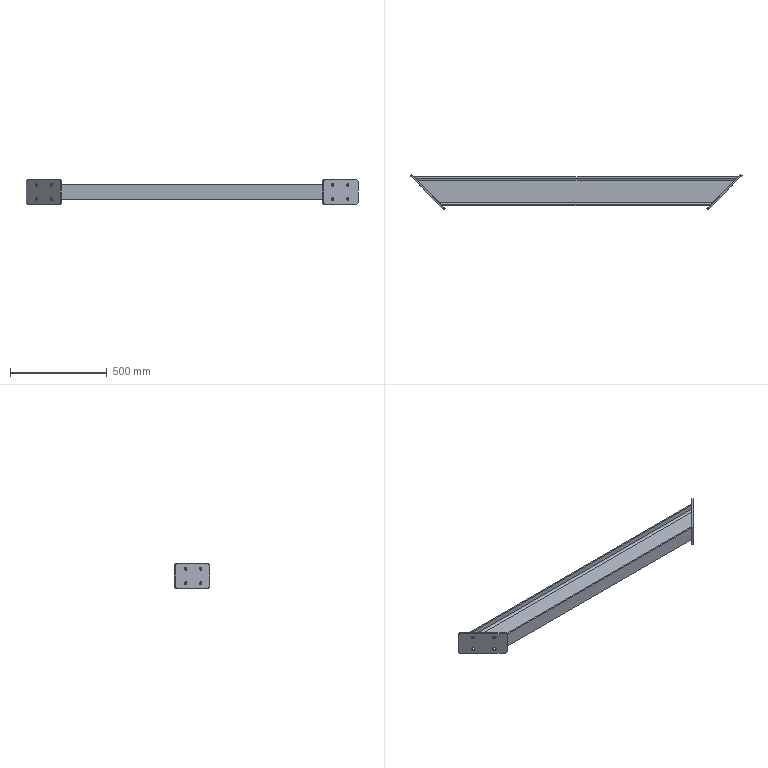Part | STEP file | PN_0059 steel column and steel beam brace 1677_Default<As Machined> | 3 solids | 46 faces | box 1715 x 182.434 x 125 mm | volume 3255129 mm3 | plane 26 | cylinder 20 | commonest cylinder face diameters 20 x12 18 x8